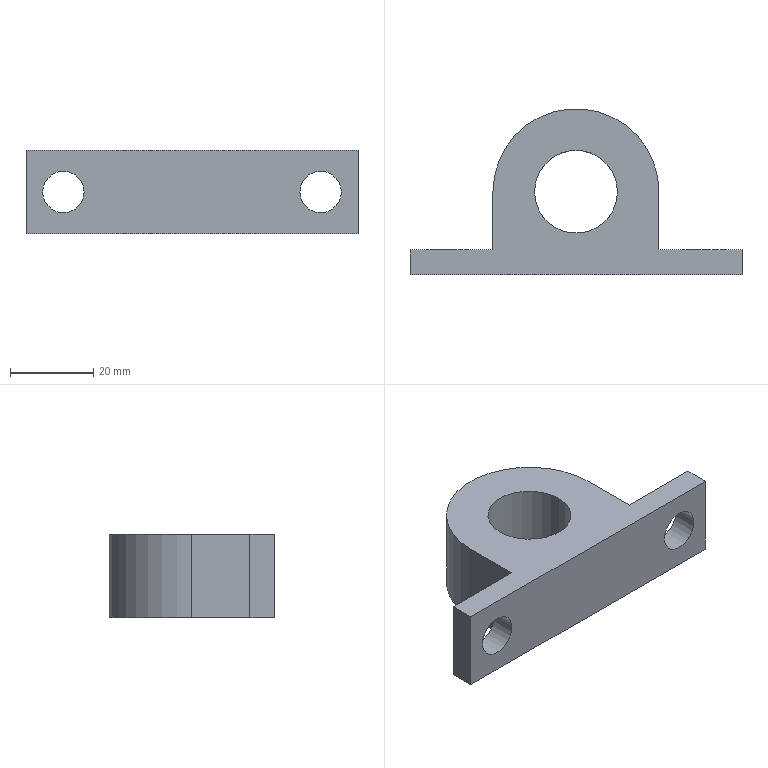Part | SolidWorks | features Extrusion 1, ICE 1 | 1 solid | 16 faces | box 80 x 40 x 20 mm | volume 26141 mm3 | plane 9 | cylinder 7 | commonest cylinder face diameters 10 x4 20 x2 40 x1
STEP:
#1=CARTESIAN_POINT('',(36.,-20.,0.));
#2=VERTEX_POINT('',#1);
#3=CARTESIAN_POINT('',(26.,-20.,0.));
#4=VERTEX_POINT('',#3);
#5=CARTESIAN_POINT('',(31.,-20.,0.));
#6=DIRECTION('',(0.,1.,0.));
#7=DIRECTION('',(-1.,0.,0.));
#8=AXIS2_PLACEMENT_3D('',#5,#6,#7);
#9=CIRCLE('',#8,5.);
#10=EDGE_CURVE('',#2,#4,#9,.T.);
#11=ORIENTED_EDGE('',*,*,#10,.F.);
#12=CARTESIAN_POINT('',(36.,-14.,0.));
#13=VERTEX_POINT('',#12);
#14=CARTESIAN_POINT('',(36.,-24.,0.));
#15=DIRECTION('',(0.,1.,0.));
#16=VECTOR('',#15,1000.);
#17=LINE('',#14,#16);
#18=EDGE_CURVE('',#2,#13,#17,.T.);
#19=ORIENTED_EDGE('',*,*,#18,.T.);
#20=CARTESIAN_POINT('',(26.,-14.,0.));
#21=VERTEX_POINT('',#20);
#22=CARTESIAN_POINT('',(31.,-14.,0.));
#23=DIRECTION('',(0.,1.,0.));
#24=DIRECTION('',(-1.,0.,0.));
#25=AXIS2_PLACEMENT_3D('',#22,#23,#24);
#26=CIRCLE('',#25,5.);
#27=EDGE_CURVE('',#13,#21,#26,.T.);
#28=ORIENTED_EDGE('',*,*,#27,.T.);
#29=CARTESIAN_POINT('',(26.,-24.,0.));
#30=DIRECTION('',(0.,1.,0.));
#31=VECTOR('',#30,1000.);
#32=LINE('',#29,#31);
#33=EDGE_CURVE('',#4,#21,#32,.T.);
#34=ORIENTED_EDGE('',*,*,#33,.F.);
#35=EDGE_LOOP('',(#11,#19,#28,#34));
#36=FACE_OUTER_BOUND('',#35,.T.);
#37=CARTESIAN_POINT('',(31.,-24.,0.));
#38=DIRECTION('',(0.,1.,0.));
#39=DIRECTION('',(-1.,0.,0.));
#40=AXIS2_PLACEMENT_3D('',#37,#38,#39);
#41=CYLINDRICAL_SURFACE('',#40,5.);
#42=ADVANCED_FACE('',(#36),#41,.F.);
#43=CARTESIAN_POINT('',(-26.,-20.,0.));
#44=VERTEX_POINT('',#43);
#45=CARTESIAN_POINT('',(-36.,-20.,0.));
#46=VERTEX_POINT('',#45);
#47=CARTESIAN_POINT('',(-31.,-20.,0.));
#48=DIRECTION('',(0.,1.,0.));
#49=DIRECTION('',(-1.,0.,0.));
#50=AXIS2_PLACEMENT_3D('',#47,#48,#49);
#51=CIRCLE('',#50,5.);
#52=EDGE_CURVE('',#44,#46,#51,.T.);
#53=ORIENTED_EDGE('',*,*,#52,.F.);
#54=CARTESIAN_POINT('',(-26.,-14.,0.));
#55=VERTEX_POINT('',#54);
#56=CARTESIAN_POINT('',(-26.,-24.,0.));
#57=DIRECTION('',(0.,1.,0.));
#58=VECTOR('',#57,1000.);
#59=LINE('',#56,#58);
#60=EDGE_CURVE('',#44,#55,#59,.T.);
#61=ORIENTED_EDGE('',*,*,#60,.T.);
#62=CARTESIAN_POINT('',(-36.,-14.,0.));
#63=VERTEX_POINT('',#62);
#64=CARTESIAN_POINT('',(-31.,-14.,0.));
#65=DIRECTION('',(0.,1.,0.));
#66=DIRECTION('',(-1.,0.,0.));
#67=AXIS2_PLACEMENT_3D('',#64,#65,#66);
#68=CIRCLE('',#67,5.);
#69=EDGE_CURVE('',#55,#63,#68,.T.);
#70=ORIENTED_EDGE('',*,*,#69,.T.);
#71=CARTESIAN_POINT('',(-36.,-24.,0.));
#72=DIRECTION('',(0.,1.,0.));
#73=VECTOR('',#72,1000.);
#74=LINE('',#71,#73);
#75=EDGE_CURVE('',#46,#63,#74,.T.);
#76=ORIENTED_EDGE('',*,*,#75,.F.);
#77=EDGE_LOOP('',(#53,#61,#70,#76));
#78=FACE_OUTER_BOUND('',#77,.T.);
#79=CARTESIAN_POINT('',(-31.,-24.,0.));
#80=DIRECTION('',(0.,1.,0.));
#81=DIRECTION('',(-1.,0.,0.));
#82=AXIS2_PLACEMENT_3D('',#79,#80,#81);
#83=CYLINDRICAL_SURFACE('',#82,5.);
#84=ADVANCED_FACE('',(#78),#83,.F.);
#85=CARTESIAN_POINT('',(-10.,0.,10.));
#86=VERTEX_POINT('',#85);
#87=CARTESIAN_POINT('',(10.,0.,10.));
#88=VERTEX_POINT('',#87);
#89=CARTESIAN_POINT('',(0.,0.,10.));
#90=DIRECTION('',(0.,0.,1.));
#91=DIRECTION('',(1.,0.,0.));
#92=AXIS2_PLACEMENT_3D('',#89,#90,#91);
#93=CIRCLE('',#92,10.);
#94=EDGE_CURVE('',#86,#88,#93,.T.);
#95=ORIENTED_EDGE('',*,*,#94,.T.);
#96=CARTESIAN_POINT('',(10.,0.,-10.));
#97=VERTEX_POINT('',#96);
#98=CARTESIAN_POINT('',(10.,0.,10.));
#99=DIRECTION('',(0.,0.,-1.));
#100=VECTOR('',#99,1000.);
#101=LINE('',#98,#100);
#102=EDGE_CURVE('',#88,#97,#101,.T.);
#103=ORIENTED_EDGE('',*,*,#102,.T.);
#104=CARTESIAN_POINT('',(-10.,0.,-10.));
#105=VERTEX_POINT('',#104);
#106=CARTESIAN_POINT('',(0.,0.,-10.));
#107=DIRECTION('',(0.,0.,1.));
#108=DIRECTION('',(1.,0.,0.));
#109=AXIS2_PLACEMENT_3D('',#106,#107,#108);
#110=CIRCLE('',#109,10.);
#111=EDGE_CURVE('',#105,#97,#110,.T.);
#112=ORIENTED_EDGE('',*,*,#111,.F.);
#113=CARTESIAN_POINT('',(-10.,0.,10.));
#114=DIRECTION('',(0.,0.,-1.));
#115=VECTOR('',#114,1000.);
#116=LINE('',#113,#115);
#117=EDGE_CURVE('',#86,#105,#116,.T.);
#118=ORIENTED_EDGE('',*,*,#117,.F.);
#119=EDGE_LOOP('',(#95,#103,#112,#118));
#120=FACE_OUTER_BOUND('',#119,.T.);
#121=CARTESIAN_POINT('',(0.,0.,10.));
#122=DIRECTION('',(0.,0.,-1.));
#123=DIRECTION('',(-1.,0.,0.));
#124=AXIS2_PLACEMENT_3D('',#121,#122,#123);
#125=CYLINDRICAL_SURFACE('',#124,10.);
#126=ADVANCED_FACE('',(#120),#125,.F.);
#127=CARTESIAN_POINT('',(-40.,-20.,-10.));
#128=VERTEX_POINT('',#127);
#129=CARTESIAN_POINT('',(-40.,-14.,-10.));
#130=VERTEX_POINT('',#129);
#131=CARTESIAN_POINT('',(-40.,0.,-10.));
#132=DIRECTION('',(0.,1.,0.));
#133=VECTOR('',#132,1000.);
#134=LINE('',#131,#133);
#135=EDGE_CURVE('',#128,#130,#134,.T.);
#136=ORIENTED_EDGE('',*,*,#135,.F.);
#137=CARTESIAN_POINT('',(-40.,-20.,10.));
#138=VERTEX_POINT('',#137);
#139=CARTESIAN_POINT('',(-40.,-20.,10.));
#140=DIRECTION('',(0.,0.,-1.));
#141=VECTOR('',#140,1000.);
#142=LINE('',#139,#141);
#143=EDGE_CURVE('',#138,#128,#142,.T.);
#144=ORIENTED_EDGE('',*,*,#143,.F.);
#145=CARTESIAN_POINT('',(-40.,-14.,10.));
#146=VERTEX_POINT('',#145);
#147=CARTESIAN_POINT('',(-40.,0.,10.));
#148=DIRECTION('',(0.,1.,0.));
#149=VECTOR('',#148,1000.);
#150=LINE('',#147,#149);
#151=EDGE_CURVE('',#138,#146,#150,.T.);
#152=ORIENTED_EDGE('',*,*,#151,.T.);
#153=CARTESIAN_POINT('',(-40.,-14.,10.));
#154=DIRECTION('',(0.,0.,-1.));
#155=VECTOR('',#154,1000.);
#156=LINE('',#153,#155);
#157=EDGE_CURVE('',#146,#130,#156,.T.);
#158=ORIENTED_EDGE('',*,*,#157,.T.);
#159=EDGE_LOOP('',(#136,#144,#152,#158));
#160=FACE_OUTER_BOUND('',#159,.T.);
#161=CARTESIAN_POINT('',(-40.,0.,10.));
#162=DIRECTION('',(-1.,0.,0.));
#163=DIRECTION('',(0.,0.,1.));
#164=AXIS2_PLACEMENT_3D('',#161,#162,#163);
#165=PLANE('',#164);
#166=ADVANCED_FACE('',(#160),#165,.T.);
#167=CARTESIAN_POINT('',(31.,-20.,0.));
#168=DIRECTION('',(0.,1.,0.));
#169=DIRECTION('',(-1.,0.,0.));
#170=AXIS2_PLACEMENT_3D('',#167,#168,#169);
#171=CIRCLE('',#170,5.);
#172=EDGE_CURVE('',#4,#2,#171,.T.);
#173=ORIENTED_EDGE('',*,*,#172,.T.);
#174=ORIENTED_EDGE('',*,*,#10,.T.);
#175=EDGE_LOOP('',(#173,#174));
#176=FACE_BOUND('',#175,.T.);
#177=CARTESIAN_POINT('',(-31.,-20.,0.));
#178=DIRECTION('',(0.,1.,0.));
#179=DIRECTION('',(-1.,0.,0.));
#180=AXIS2_PLACEMENT_3D('',#177,#178,#179);
#181=CIRCLE('',#180,5.);
#182=EDGE_CURVE('',#46,#44,#181,.T.);
#183=ORIENTED_EDGE('',*,*,#182,.T.);
#184=ORIENTED_EDGE('',*,*,#52,.T.);
#185=EDGE_LOOP('',(#183,#184));
#186=FACE_BOUND('',#185,.T.);
#187=CARTESIAN_POINT('',(40.,-20.,-10.));
#188=VERTEX_POINT('',#187);
#189=CARTESIAN_POINT('',(0.,-20.,-10.));
#190=DIRECTION('',(1.,0.,0.));
#191=VECTOR('',#190,1000.);
#192=LINE('',#189,#191);
#193=EDGE_CURVE('',#128,#188,#192,.T.);
#194=ORIENTED_EDGE('',*,*,#193,.T.);
#195=CARTESIAN_POINT('',(40.,-20.,10.));
#196=VERTEX_POINT('',#195);
#197=CARTESIAN_POINT('',(40.,-20.,10.));
#198=DIRECTION('',(0.,0.,-1.));
#199=VECTOR('',#198,1000.);
#200=LINE('',#197,#199);
#201=EDGE_CURVE('',#196,#188,#200,.T.);
#202=ORIENTED_EDGE('',*,*,#201,.F.);
#203=CARTESIAN_POINT('',(0.,-20.,10.));
#204=DIRECTION('',(1.,0.,0.));
#205=VECTOR('',#204,1000.);
#206=LINE('',#203,#205);
#207=EDGE_CURVE('',#138,#196,#206,.T.);
#208=ORIENTED_EDGE('',*,*,#207,.F.);
#209=ORIENTED_EDGE('',*,*,#143,.T.);
#210=EDGE_LOOP('',(#194,#202,#208,#209));
#211=FACE_OUTER_BOUND('',#210,.T.);
#212=CARTESIAN_POINT('',(0.,-20.,10.));
#213=DIRECTION('',(0.,1.,0.));
#214=DIRECTION('',(-1.,0.,0.));
#215=AXIS2_PLACEMENT_3D('',#212,#213,#214);
#216=PLANE('',#215);
#217=ADVANCED_FACE('',(#176,#186,#211),#216,.F.);
#218=CARTESIAN_POINT('',(40.,-14.,-10.));
#219=VERTEX_POINT('',#218);
#220=CARTESIAN_POINT('',(40.,0.,-10.));
#221=DIRECTION('',(0.,-1.,0.));
#222=VECTOR('',#221,1000.);
#223=LINE('',#220,#222);
#224=EDGE_CURVE('',#219,#188,#223,.T.);
#225=ORIENTED_EDGE('',*,*,#224,.F.);
#226=CARTESIAN_POINT('',(40.,-14.,10.));
#227=VERTEX_POINT('',#226);
#228=CARTESIAN_POINT('',(40.,-14.,10.));
#229=DIRECTION('',(0.,0.,-1.));
#230=VECTOR('',#229,1000.);
#231=LINE('',#228,#230);
#232=EDGE_CURVE('',#227,#219,#231,.T.);
#233=ORIENTED_EDGE('',*,*,#232,.F.);
#234=CARTESIAN_POINT('',(40.,0.,10.));
#235=DIRECTION('',(0.,-1.,0.));
#236=VECTOR('',#235,1000.);
#237=LINE('',#234,#236);
#238=EDGE_CURVE('',#227,#196,#237,.T.);
#239=ORIENTED_EDGE('',*,*,#238,.T.);
#240=ORIENTED_EDGE('',*,*,#201,.T.);
#241=EDGE_LOOP('',(#225,#233,#239,#240));
#242=FACE_OUTER_BOUND('',#241,.T.);
#243=CARTESIAN_POINT('',(40.,0.,10.));
#244=DIRECTION('',(1.,0.,0.));
#245=DIRECTION('',(0.,0.,-1.));
#246=AXIS2_PLACEMENT_3D('',#243,#244,#245);
#247=PLANE('',#246);
#248=ADVANCED_FACE('',(#242),#247,.T.);
#249=CARTESIAN_POINT('',(31.,-14.,0.));
#250=DIRECTION('',(0.,1.,0.));
#251=DIRECTION('',(-1.,0.,0.));
#252=AXIS2_PLACEMENT_3D('',#249,#250,#251);
#253=CIRCLE('',#252,5.);
#254=EDGE_CURVE('',#21,#13,#253,.T.);
#255=ORIENTED_EDGE('',*,*,#254,.F.);
#256=ORIENTED_EDGE('',*,*,#27,.F.);
#257=EDGE_LOOP('',(#255,#256));
#258=FACE_BOUND('',#257,.T.);
#259=CARTESIAN_POINT('',(20.,-14.,-10.));
#260=VERTEX_POINT('',#259);
#261=CARTESIAN_POINT('',(0.,-14.,-10.));
#262=DIRECTION('',(1.,0.,0.));
#263=VECTOR('',#262,1000.);
#264=LINE('',#261,#263);
#265=EDGE_CURVE('',#260,#219,#264,.T.);
#266=ORIENTED_EDGE('',*,*,#265,.F.);
#267=CARTESIAN_POINT('',(20.,-14.,10.));
#268=VERTEX_POINT('',#267);
#269=CARTESIAN_POINT('',(20.,-14.,10.));
#270=DIRECTION('',(0.,0.,-1.));
#271=VECTOR('',#270,1000.);
#272=LINE('',#269,#271);
#273=EDGE_CURVE('',#268,#260,#272,.T.);
#274=ORIENTED_EDGE('',*,*,#273,.F.);
#275=CARTESIAN_POINT('',(0.,-14.,10.));
#276=DIRECTION('',(1.,0.,0.));
#277=VECTOR('',#276,1000.);
#278=LINE('',#275,#277);
#279=EDGE_CURVE('',#268,#227,#278,.T.);
#280=ORIENTED_EDGE('',*,*,#279,.T.);
#281=ORIENTED_EDGE('',*,*,#232,.T.);
#282=EDGE_LOOP('',(#266,#274,#280,#281));
#283=FACE_OUTER_BOUND('',#282,.T.);
#284=CARTESIAN_POINT('',(0.,-14.,10.));
#285=DIRECTION('',(0.,1.,0.));
#286=DIRECTION('',(-1.,0.,0.));
#287=AXIS2_PLACEMENT_3D('',#284,#285,#286);
#288=PLANE('',#287);
#289=ADVANCED_FACE('',(#258,#283),#288,.T.);
#290=CARTESIAN_POINT('',(20.,0.,-10.));
#291=VERTEX_POINT('',#290);
#292=CARTESIAN_POINT('',(20.,0.,-10.));
#293=DIRECTION('',(0.,-1.,0.));
#294=VECTOR('',#293,1000.);
#295=LINE('',#292,#294);
#296=EDGE_CURVE('',#291,#260,#295,.T.);
#297=ORIENTED_EDGE('',*,*,#296,.F.);
#298=CARTESIAN_POINT('',(20.,0.,10.));
#299=VERTEX_POINT('',#298);
#300=CARTESIAN_POINT('',(20.,0.,10.));
#301=DIRECTION('',(0.,0.,-1.));
#302=VECTOR('',#301,1000.);
#303=LINE('',#300,#302);
#304=EDGE_CURVE('',#299,#291,#303,.T.);
#305=ORIENTED_EDGE('',*,*,#304,.F.);
#306=CARTESIAN_POINT('',(20.,0.,10.));
#307=DIRECTION('',(0.,-1.,0.));
#308=VECTOR('',#307,1000.);
#309=LINE('',#306,#308);
#310=EDGE_CURVE('',#299,#268,#309,.T.);
#311=ORIENTED_EDGE('',*,*,#310,.T.);
#312=ORIENTED_EDGE('',*,*,#273,.T.);
#313=EDGE_LOOP('',(#297,#305,#311,#312));
#314=FACE_OUTER_BOUND('',#313,.T.);
#315=CARTESIAN_POINT('',(20.,0.,10.));
#316=DIRECTION('',(1.,0.,0.));
#317=DIRECTION('',(0.,0.,-1.));
#318=AXIS2_PLACEMENT_3D('',#315,#316,#317);
#319=PLANE('',#318);
#320=ADVANCED_FACE('',(#314),#319,.T.);
#321=CARTESIAN_POINT('',(-20.,0.,-10.));
#322=VERTEX_POINT('',#321);
#323=CARTESIAN_POINT('',(0.,0.,-10.));
#324=DIRECTION('',(0.,0.,1.));
#325=DIRECTION('',(1.,0.,0.));
#326=AXIS2_PLACEMENT_3D('',#323,#324,#325);
#327=CIRCLE('',#326,20.);
#328=EDGE_CURVE('',#291,#322,#327,.T.);
#329=ORIENTED_EDGE('',*,*,#328,.T.);
#330=CARTESIAN_POINT('',(-20.,0.,10.));
#331=VERTEX_POINT('',#330);
#332=CARTESIAN_POINT('',(-20.,0.,10.));
#333=DIRECTION('',(0.,0.,-1.));
#334=VECTOR('',#333,1000.);
#335=LINE('',#332,#334);
#336=EDGE_CURVE('',#331,#322,#335,.T.);
#337=ORIENTED_EDGE('',*,*,#336,.F.);
#338=CARTESIAN_POINT('',(0.,0.,10.));
#339=DIRECTION('',(0.,0.,1.));
#340=DIRECTION('',(1.,0.,0.));
#341=AXIS2_PLACEMENT_3D('',#338,#339,#340);
#342=CIRCLE('',#341,20.);
#343=EDGE_CURVE('',#299,#331,#342,.T.);
#344=ORIENTED_EDGE('',*,*,#343,.F.);
#345=ORIENTED_EDGE('',*,*,#304,.T.);
#346=EDGE_LOOP('',(#329,#337,#344,#345));
#347=FACE_OUTER_BOUND('',#346,.T.);
#348=CARTESIAN_POINT('',(0.,0.,10.));
#349=DIRECTION('',(0.,0.,-1.));
#350=DIRECTION('',(-1.,0.,0.));
#351=AXIS2_PLACEMENT_3D('',#348,#349,#350);
#352=CYLINDRICAL_SURFACE('',#351,20.);
#353=ADVANCED_FACE('',(#347),#352,.T.);
#354=CARTESIAN_POINT('',(-20.,-14.,-10.));
#355=VERTEX_POINT('',#354);
#356=CARTESIAN_POINT('',(-20.,0.,-10.));
#357=DIRECTION('',(0.,-1.,0.));
#358=VECTOR('',#357,1000.);
#359=LINE('',#356,#358);
#360=EDGE_CURVE('',#322,#355,#359,.T.);
#361=ORIENTED_EDGE('',*,*,#360,.T.);
#362=CARTESIAN_POINT('',(-20.,-14.,10.));
#363=VERTEX_POINT('',#362);
#364=CARTESIAN_POINT('',(-20.,-14.,10.));
#365=DIRECTION('',(0.,0.,-1.));
#366=VECTOR('',#365,1000.);
#367=LINE('',#364,#366);
#368=EDGE_CURVE('',#363,#355,#367,.T.);
#369=ORIENTED_EDGE('',*,*,#368,.F.);
#370=CARTESIAN_POINT('',(-20.,0.,10.));
#371=DIRECTION('',(0.,-1.,0.));
#372=VECTOR('',#371,1000.);
#373=LINE('',#370,#372);
#374=EDGE_CURVE('',#331,#363,#373,.T.);
#375=ORIENTED_EDGE('',*,*,#374,.F.);
#376=ORIENTED_EDGE('',*,*,#336,.T.);
#377=EDGE_LOOP('',(#361,#369,#375,#376));
#378=FACE_OUTER_BOUND('',#377,.T.);
#379=CARTESIAN_POINT('',(-20.,0.,10.));
#380=DIRECTION('',(1.,0.,0.));
#381=DIRECTION('',(0.,0.,-1.));
#382=AXIS2_PLACEMENT_3D('',#379,#380,#381);
#383=PLANE('',#382);
#384=ADVANCED_FACE('',(#378),#383,.F.);
#385=CARTESIAN_POINT('',(-31.,-14.,0.));
#386=DIRECTION('',(0.,1.,0.));
#387=DIRECTION('',(-1.,0.,0.));
#388=AXIS2_PLACEMENT_3D('',#385,#386,#387);
#389=CIRCLE('',#388,5.);
#390=EDGE_CURVE('',#63,#55,#389,.T.);
#391=ORIENTED_EDGE('',*,*,#390,.F.);
#392=ORIENTED_EDGE('',*,*,#69,.F.);
#393=EDGE_LOOP('',(#391,#392));
#394=FACE_BOUND('',#393,.T.);
#395=CARTESIAN_POINT('',(0.,-14.,-10.));
#396=DIRECTION('',(1.,0.,0.));
#397=VECTOR('',#396,1000.);
#398=LINE('',#395,#397);
#399=EDGE_CURVE('',#130,#355,#398,.T.);
#400=ORIENTED_EDGE('',*,*,#399,.F.);
#401=ORIENTED_EDGE('',*,*,#157,.F.);
#402=CARTESIAN_POINT('',(0.,-14.,10.));
#403=DIRECTION('',(1.,0.,0.));
#404=VECTOR('',#403,1000.);
#405=LINE('',#402,#404);
#406=EDGE_CURVE('',#146,#363,#405,.T.);
#407=ORIENTED_EDGE('',*,*,#406,.T.);
#408=ORIENTED_EDGE('',*,*,#368,.T.);
#409=EDGE_LOOP('',(#400,#401,#407,#408));
#410=FACE_OUTER_BOUND('',#409,.T.);
#411=CARTESIAN_POINT('',(0.,-14.,10.));
#412=DIRECTION('',(0.,1.,0.));
#413=DIRECTION('',(-1.,0.,0.));
#414=AXIS2_PLACEMENT_3D('',#411,#412,#413);
#415=PLANE('',#414);
#416=ADVANCED_FACE('',(#394,#410),#415,.T.);
#417=ORIENTED_EDGE('',*,*,#102,.F.);
#418=CARTESIAN_POINT('',(0.,0.,10.));
#419=DIRECTION('',(0.,0.,1.));
#420=DIRECTION('',(1.,0.,0.));
#421=AXIS2_PLACEMENT_3D('',#418,#419,#420);
#422=CIRCLE('',#421,10.);
#423=EDGE_CURVE('',#88,#86,#422,.T.);
#424=ORIENTED_EDGE('',*,*,#423,.T.);
#425=ORIENTED_EDGE('',*,*,#117,.T.);
#426=CARTESIAN_POINT('',(0.,0.,-10.));
#427=DIRECTION('',(0.,0.,1.));
#428=DIRECTION('',(1.,0.,0.));
#429=AXIS2_PLACEMENT_3D('',#426,#427,#428);
#430=CIRCLE('',#429,10.);
#431=EDGE_CURVE('',#97,#105,#430,.T.);
#432=ORIENTED_EDGE('',*,*,#431,.F.);
#433=EDGE_LOOP('',(#417,#424,#425,#432));
#434=FACE_OUTER_BOUND('',#433,.T.);
#435=CARTESIAN_POINT('',(0.,0.,10.));
#436=DIRECTION('',(0.,0.,-1.));
#437=DIRECTION('',(-1.,0.,0.));
#438=AXIS2_PLACEMENT_3D('',#435,#436,#437);
#439=CYLINDRICAL_SURFACE('',#438,10.);
#440=ADVANCED_FACE('',(#434),#439,.F.);
#441=ORIENTED_EDGE('',*,*,#151,.F.);
#442=ORIENTED_EDGE('',*,*,#207,.T.);
#443=ORIENTED_EDGE('',*,*,#238,.F.);
#444=ORIENTED_EDGE('',*,*,#279,.F.);
#445=ORIENTED_EDGE('',*,*,#310,.F.);
#446=ORIENTED_EDGE('',*,*,#343,.T.);
#447=ORIENTED_EDGE('',*,*,#374,.T.);
#448=ORIENTED_EDGE('',*,*,#406,.F.);
#449=EDGE_LOOP('',(#441,#442,#443,#444,#445,#446,#447,#448));
#450=FACE_OUTER_BOUND('',#449,.T.);
#451=ORIENTED_EDGE('',*,*,#94,.F.);
#452=ORIENTED_EDGE('',*,*,#423,.F.);
#453=EDGE_LOOP('',(#451,#452));
#454=FACE_BOUND('',#453,.T.);
#455=CARTESIAN_POINT('',(0.,0.,10.));
#456=DIRECTION('',(0.,0.,1.));
#457=DIRECTION('',(1.,0.,0.));
#458=AXIS2_PLACEMENT_3D('',#455,#456,#457);
#459=PLANE('',#458);
#460=ADVANCED_FACE('',(#450,#454),#459,.T.);
#461=ORIENTED_EDGE('',*,*,#135,.T.);
#462=ORIENTED_EDGE('',*,*,#399,.T.);
#463=ORIENTED_EDGE('',*,*,#360,.F.);
#464=ORIENTED_EDGE('',*,*,#328,.F.);
#465=ORIENTED_EDGE('',*,*,#296,.T.);
#466=ORIENTED_EDGE('',*,*,#265,.T.);
#467=ORIENTED_EDGE('',*,*,#224,.T.);
#468=ORIENTED_EDGE('',*,*,#193,.F.);
#469=EDGE_LOOP('',(#461,#462,#463,#464,#465,#466,#467,#468));
#470=FACE_OUTER_BOUND('',#469,.T.);
#471=ORIENTED_EDGE('',*,*,#111,.T.);
#472=ORIENTED_EDGE('',*,*,#431,.T.);
#473=EDGE_LOOP('',(#471,#472));
#474=FACE_BOUND('',#473,.T.);
#475=CARTESIAN_POINT('',(0.,0.,-10.));
#476=DIRECTION('',(0.,0.,1.));
#477=DIRECTION('',(1.,0.,0.));
#478=AXIS2_PLACEMENT_3D('',#475,#476,#477);
#479=PLANE('',#478);
#480=ADVANCED_FACE('',(#470,#474),#479,.F.);
#481=ORIENTED_EDGE('',*,*,#60,.F.);
#482=ORIENTED_EDGE('',*,*,#182,.F.);
#483=ORIENTED_EDGE('',*,*,#75,.T.);
#484=ORIENTED_EDGE('',*,*,#390,.T.);
#485=EDGE_LOOP('',(#481,#482,#483,#484));
#486=FACE_OUTER_BOUND('',#485,.T.);
#487=CARTESIAN_POINT('',(-31.,-24.,0.));
#488=DIRECTION('',(0.,1.,0.));
#489=DIRECTION('',(-1.,0.,0.));
#490=AXIS2_PLACEMENT_3D('',#487,#488,#489);
#491=CYLINDRICAL_SURFACE('',#490,5.);
#492=ADVANCED_FACE('',(#486),#491,.F.);
#493=ORIENTED_EDGE('',*,*,#18,.F.);
#494=ORIENTED_EDGE('',*,*,#172,.F.);
#495=ORIENTED_EDGE('',*,*,#33,.T.);
#496=ORIENTED_EDGE('',*,*,#254,.T.);
#497=EDGE_LOOP('',(#493,#494,#495,#496));
#498=FACE_OUTER_BOUND('',#497,.T.);
#499=CARTESIAN_POINT('',(31.,-24.,0.));
#500=DIRECTION('',(0.,1.,0.));
#501=DIRECTION('',(-1.,0.,0.));
#502=AXIS2_PLACEMENT_3D('',#499,#500,#501);
#503=CYLINDRICAL_SURFACE('',#502,5.);
#504=ADVANCED_FACE('',(#498),#503,.F.);
#505=CLOSED_SHELL('',(#42,#84,#126,#166,#217,#248,#289,#320,#353,#384,#416,#440,#460,#480,#492,#504));
#506=MANIFOLD_SOLID_BREP('',#505);
#507=CARTESIAN_POINT('',(0.,0.,0.));
#508=DIRECTION('',(0.,0.,1.));
#509=DIRECTION('',(1.,0.,0.));
#510=AXIS2_PLACEMENT_3D('',#507,#508,#509);
#511=(LENGTH_UNIT()NAMED_UNIT(*)SI_UNIT(.MILLI.,.METRE.));
#512=UNCERTAINTY_MEASURE_WITH_UNIT(LENGTH_MEASURE(0.00001),#511,'','');
#513=(NAMED_UNIT(*)PLANE_ANGLE_UNIT()SI_UNIT($,.RADIAN.));
#514=(NAMED_UNIT(*)SI_UNIT($,.STERADIAN.)SOLID_ANGLE_UNIT());
#515=(GEOMETRIC_REPRESENTATION_CONTEXT(3)GLOBAL_UNCERTAINTY_ASSIGNED_CONTEXT((#512))GLOBAL_UNIT_ASSIGNED_CONTEXT((#511,#513,#514))REPRESENTATION_CONTEXT('',''));
#516=ADVANCED_BREP_SHAPE_REPRESENTATION('',(#506,#510),#515);